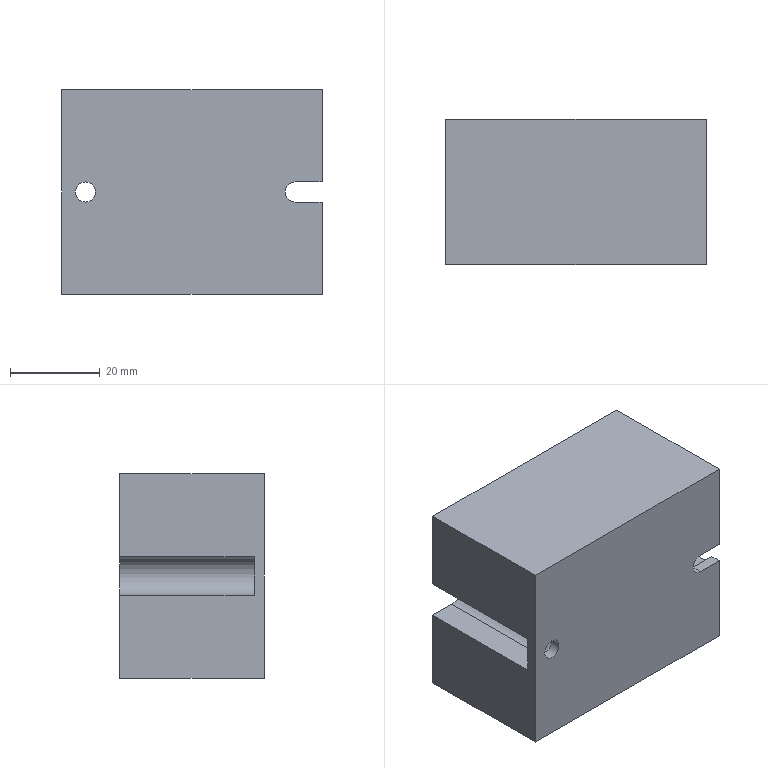Part | NX | features BREP 1 | 1 solid | 19 faces | box 58 x 32.3 x 45.5 mm | volume 80360 mm3 | plane 15 | cylinder 4 | commonest cylinder face diameters 4.5 x2 8.5 x2
STEP:
#1=CARTESIAN_POINT('',(-23.75,2.3,2.25));
#2=VERTEX_POINT('',#1);
#3=CARTESIAN_POINT('',(-23.75,2.3,0.));
#4=DIRECTION('',(0.,1.,0.));
#5=DIRECTION('',(0.,0.,1.));
#6=AXIS2_PLACEMENT_3D('',#3,#4,#5);
#7=CIRCLE('',#6,2.25);
#8=EDGE_CURVE('',#2,#2,#7,.T.);
#9=ORIENTED_EDGE('',*,*,#8,.T.);
#10=EDGE_LOOP('',(#9));
#11=FACE_BOUND('',#10,.T.);
#12=CARTESIAN_POINT('',(-23.75,0.,2.25));
#13=VERTEX_POINT('',#12);
#14=CARTESIAN_POINT('',(-23.75,0.,0.));
#15=DIRECTION('',(0.,1.,0.));
#16=DIRECTION('',(0.,0.,1.));
#17=AXIS2_PLACEMENT_3D('',#14,#15,#16);
#18=CIRCLE('',#17,2.25);
#19=EDGE_CURVE('',#13,#13,#18,.T.);
#20=ORIENTED_EDGE('',*,*,#19,.F.);
#21=EDGE_LOOP('',(#20));
#22=FACE_BOUND('',#21,.T.);
#23=CARTESIAN_POINT('',(-23.75,-27.7,0.));
#24=DIRECTION('',(0.,1.,0.));
#25=DIRECTION('',(0.,0.,1.));
#26=AXIS2_PLACEMENT_3D('',#23,#24,#25);
#27=CYLINDRICAL_SURFACE('',#26,2.25);
#28=ADVANCED_FACE('',(#11,#22),#27,.F.);
#29=CARTESIAN_POINT('',(29.,2.3,-2.25));
#30=VERTEX_POINT('',#29);
#31=CARTESIAN_POINT('',(29.,2.3,-4.25));
#32=VERTEX_POINT('',#31);
#33=CARTESIAN_POINT('',(29.,2.3,-22.75));
#34=DIRECTION('',(0.,0.,-1.));
#35=VECTOR('',#34,1000.);
#36=LINE('',#33,#35);
#37=EDGE_CURVE('',#30,#32,#36,.T.);
#38=ORIENTED_EDGE('',*,*,#37,.F.);
#39=CARTESIAN_POINT('',(29.,0.,-2.25));
#40=VERTEX_POINT('',#39);
#41=CARTESIAN_POINT('',(29.,32.3,-2.25));
#42=DIRECTION('',(0.,-1.,0.));
#43=VECTOR('',#42,1000.);
#44=LINE('',#41,#43);
#45=EDGE_CURVE('',#30,#40,#44,.T.);
#46=ORIENTED_EDGE('',*,*,#45,.T.);
#47=CARTESIAN_POINT('',(29.,0.,-22.75));
#48=VERTEX_POINT('',#47);
#49=CARTESIAN_POINT('',(29.,0.,-22.75));
#50=DIRECTION('',(0.,0.,-1.));
#51=VECTOR('',#50,1000.);
#52=LINE('',#49,#51);
#53=EDGE_CURVE('',#40,#48,#52,.T.);
#54=ORIENTED_EDGE('',*,*,#53,.T.);
#55=CARTESIAN_POINT('',(29.,32.3,-22.75));
#56=VERTEX_POINT('',#55);
#57=CARTESIAN_POINT('',(29.,32.3,-22.75));
#58=DIRECTION('',(0.,-1.,0.));
#59=VECTOR('',#58,1000.);
#60=LINE('',#57,#59);
#61=EDGE_CURVE('',#56,#48,#60,.T.);
#62=ORIENTED_EDGE('',*,*,#61,.F.);
#63=CARTESIAN_POINT('',(29.,32.3,-4.25));
#64=VERTEX_POINT('',#63);
#65=CARTESIAN_POINT('',(29.,32.3,-22.75));
#66=DIRECTION('',(0.,0.,-1.));
#67=VECTOR('',#66,1000.);
#68=LINE('',#65,#67);
#69=EDGE_CURVE('',#64,#56,#68,.T.);
#70=ORIENTED_EDGE('',*,*,#69,.F.);
#71=CARTESIAN_POINT('',(29.,32.3,-4.25));
#72=DIRECTION('',(0.,-1.,0.));
#73=VECTOR('',#72,1000.);
#74=LINE('',#71,#73);
#75=EDGE_CURVE('',#64,#32,#74,.T.);
#76=ORIENTED_EDGE('',*,*,#75,.T.);
#77=EDGE_LOOP('',(#38,#46,#54,#62,#70,#76));
#78=FACE_BOUND('',#77,.T.);
#79=CARTESIAN_POINT('',(29.,32.3,-22.75));
#80=DIRECTION('',(-1.,0.,0.));
#81=DIRECTION('',(0.,0.,1.));
#82=AXIS2_PLACEMENT_3D('',#79,#80,#81);
#83=PLANE('',#82);
#84=ADVANCED_FACE('',(#78),#83,.F.);
#85=CARTESIAN_POINT('',(29.,0.,22.75));
#86=VERTEX_POINT('',#85);
#87=CARTESIAN_POINT('',(29.,0.,2.25));
#88=VERTEX_POINT('',#87);
#89=CARTESIAN_POINT('',(29.,0.,-22.75));
#90=DIRECTION('',(0.,0.,-1.));
#91=VECTOR('',#90,1000.);
#92=LINE('',#89,#91);
#93=EDGE_CURVE('',#86,#88,#92,.T.);
#94=ORIENTED_EDGE('',*,*,#93,.T.);
#95=CARTESIAN_POINT('',(29.,2.3,2.25));
#96=VERTEX_POINT('',#95);
#97=CARTESIAN_POINT('',(29.,32.3,2.25));
#98=DIRECTION('',(0.,1.,0.));
#99=VECTOR('',#98,1000.);
#100=LINE('',#97,#99);
#101=EDGE_CURVE('',#88,#96,#100,.T.);
#102=ORIENTED_EDGE('',*,*,#101,.T.);
#103=CARTESIAN_POINT('',(29.,2.3,4.25));
#104=VERTEX_POINT('',#103);
#105=CARTESIAN_POINT('',(29.,2.3,-22.75));
#106=DIRECTION('',(0.,0.,-1.));
#107=VECTOR('',#106,1000.);
#108=LINE('',#105,#107);
#109=EDGE_CURVE('',#104,#96,#108,.T.);
#110=ORIENTED_EDGE('',*,*,#109,.F.);
#111=CARTESIAN_POINT('',(29.,32.3,4.25));
#112=VERTEX_POINT('',#111);
#113=CARTESIAN_POINT('',(29.,32.3,4.25));
#114=DIRECTION('',(0.,1.,0.));
#115=VECTOR('',#114,1000.);
#116=LINE('',#113,#115);
#117=EDGE_CURVE('',#104,#112,#116,.T.);
#118=ORIENTED_EDGE('',*,*,#117,.T.);
#119=CARTESIAN_POINT('',(29.,32.3,22.75));
#120=VERTEX_POINT('',#119);
#121=CARTESIAN_POINT('',(29.,32.3,-22.75));
#122=DIRECTION('',(0.,0.,-1.));
#123=VECTOR('',#122,1000.);
#124=LINE('',#121,#123);
#125=EDGE_CURVE('',#120,#112,#124,.T.);
#126=ORIENTED_EDGE('',*,*,#125,.F.);
#127=CARTESIAN_POINT('',(29.,32.3,22.75));
#128=DIRECTION('',(0.,-1.,0.));
#129=VECTOR('',#128,1000.);
#130=LINE('',#127,#129);
#131=EDGE_CURVE('',#120,#86,#130,.T.);
#132=ORIENTED_EDGE('',*,*,#131,.T.);
#133=EDGE_LOOP('',(#94,#102,#110,#118,#126,#132));
#134=FACE_BOUND('',#133,.T.);
#135=CARTESIAN_POINT('',(29.,32.3,-22.75));
#136=DIRECTION('',(-1.,0.,0.));
#137=DIRECTION('',(0.,0.,1.));
#138=AXIS2_PLACEMENT_3D('',#135,#136,#137);
#139=PLANE('',#138);
#140=ADVANCED_FACE('',(#134),#139,.F.);
#141=CARTESIAN_POINT('',(-29.,0.,-22.75));
#142=VERTEX_POINT('',#141);
#143=CARTESIAN_POINT('',(-29.,0.,-22.75));
#144=DIRECTION('',(-1.,0.,0.));
#145=VECTOR('',#144,1000.);
#146=LINE('',#143,#145);
#147=EDGE_CURVE('',#48,#142,#146,.T.);
#148=ORIENTED_EDGE('',*,*,#147,.T.);
#149=CARTESIAN_POINT('',(-29.,32.3,-22.75));
#150=VERTEX_POINT('',#149);
#151=CARTESIAN_POINT('',(-29.,32.3,-22.75));
#152=DIRECTION('',(0.,-1.,0.));
#153=VECTOR('',#152,1000.);
#154=LINE('',#151,#153);
#155=EDGE_CURVE('',#150,#142,#154,.T.);
#156=ORIENTED_EDGE('',*,*,#155,.F.);
#157=CARTESIAN_POINT('',(-29.,32.3,-22.75));
#158=DIRECTION('',(-1.,0.,0.));
#159=VECTOR('',#158,1000.);
#160=LINE('',#157,#159);
#161=EDGE_CURVE('',#56,#150,#160,.T.);
#162=ORIENTED_EDGE('',*,*,#161,.F.);
#163=ORIENTED_EDGE('',*,*,#61,.T.);
#164=EDGE_LOOP('',(#148,#156,#162,#163));
#165=FACE_BOUND('',#164,.T.);
#166=CARTESIAN_POINT('',(-29.,32.3,-22.75));
#167=DIRECTION('',(0.,0.,1.));
#168=DIRECTION('',(1.,0.,0.));
#169=AXIS2_PLACEMENT_3D('',#166,#167,#168);
#170=PLANE('',#169);
#171=ADVANCED_FACE('',(#165),#170,.F.);
#172=CARTESIAN_POINT('',(-29.,32.3,4.25));
#173=VERTEX_POINT('',#172);
#174=CARTESIAN_POINT('',(-29.,32.3,22.75));
#175=VERTEX_POINT('',#174);
#176=CARTESIAN_POINT('',(-29.,32.3,-22.75));
#177=DIRECTION('',(0.,0.,1.));
#178=VECTOR('',#177,1000.);
#179=LINE('',#176,#178);
#180=EDGE_CURVE('',#173,#175,#179,.T.);
#181=ORIENTED_EDGE('',*,*,#180,.F.);
#182=CARTESIAN_POINT('',(-29.,2.3,4.25));
#183=VERTEX_POINT('',#182);
#184=CARTESIAN_POINT('',(-29.,32.3,4.25));
#185=DIRECTION('',(0.,-1.,0.));
#186=VECTOR('',#185,1000.);
#187=LINE('',#184,#186);
#188=EDGE_CURVE('',#173,#183,#187,.T.);
#189=ORIENTED_EDGE('',*,*,#188,.T.);
#190=CARTESIAN_POINT('',(-29.,2.3,-4.25));
#191=VERTEX_POINT('',#190);
#192=CARTESIAN_POINT('',(-29.,2.3,-22.75));
#193=DIRECTION('',(0.,0.,-1.));
#194=VECTOR('',#193,1000.);
#195=LINE('',#192,#194);
#196=EDGE_CURVE('',#183,#191,#195,.T.);
#197=ORIENTED_EDGE('',*,*,#196,.T.);
#198=CARTESIAN_POINT('',(-29.,32.3,-4.25));
#199=VERTEX_POINT('',#198);
#200=CARTESIAN_POINT('',(-29.,32.3,-4.25));
#201=DIRECTION('',(0.,1.,0.));
#202=VECTOR('',#201,1000.);
#203=LINE('',#200,#202);
#204=EDGE_CURVE('',#191,#199,#203,.T.);
#205=ORIENTED_EDGE('',*,*,#204,.T.);
#206=CARTESIAN_POINT('',(-29.,32.3,-22.75));
#207=DIRECTION('',(0.,0.,1.));
#208=VECTOR('',#207,1000.);
#209=LINE('',#206,#208);
#210=EDGE_CURVE('',#150,#199,#209,.T.);
#211=ORIENTED_EDGE('',*,*,#210,.F.);
#212=ORIENTED_EDGE('',*,*,#155,.T.);
#213=CARTESIAN_POINT('',(-29.,0.,22.75));
#214=VERTEX_POINT('',#213);
#215=CARTESIAN_POINT('',(-29.,0.,-22.75));
#216=DIRECTION('',(0.,0.,1.));
#217=VECTOR('',#216,1000.);
#218=LINE('',#215,#217);
#219=EDGE_CURVE('',#142,#214,#218,.T.);
#220=ORIENTED_EDGE('',*,*,#219,.T.);
#221=CARTESIAN_POINT('',(-29.,32.3,22.75));
#222=DIRECTION('',(0.,-1.,0.));
#223=VECTOR('',#222,1000.);
#224=LINE('',#221,#223);
#225=EDGE_CURVE('',#175,#214,#224,.T.);
#226=ORIENTED_EDGE('',*,*,#225,.F.);
#227=EDGE_LOOP('',(#181,#189,#197,#205,#211,#212,#220,#226));
#228=FACE_BOUND('',#227,.T.);
#229=CARTESIAN_POINT('',(-29.,32.3,-22.75));
#230=DIRECTION('',(1.,0.,0.));
#231=DIRECTION('',(0.,0.,-1.));
#232=AXIS2_PLACEMENT_3D('',#229,#230,#231);
#233=PLANE('',#232);
#234=ADVANCED_FACE('',(#228),#233,.F.);
#235=CARTESIAN_POINT('',(-29.,0.,22.75));
#236=DIRECTION('',(1.,0.,0.));
#237=VECTOR('',#236,1000.);
#238=LINE('',#235,#237);
#239=EDGE_CURVE('',#214,#86,#238,.T.);
#240=ORIENTED_EDGE('',*,*,#239,.T.);
#241=ORIENTED_EDGE('',*,*,#131,.F.);
#242=CARTESIAN_POINT('',(-29.,32.3,22.75));
#243=DIRECTION('',(1.,0.,0.));
#244=VECTOR('',#243,1000.);
#245=LINE('',#242,#244);
#246=EDGE_CURVE('',#175,#120,#245,.T.);
#247=ORIENTED_EDGE('',*,*,#246,.F.);
#248=ORIENTED_EDGE('',*,*,#225,.T.);
#249=EDGE_LOOP('',(#240,#241,#247,#248));
#250=FACE_BOUND('',#249,.T.);
#251=CARTESIAN_POINT('',(-29.,32.3,22.75));
#252=DIRECTION('',(0.,0.,-1.));
#253=DIRECTION('',(-1.,0.,0.));
#254=AXIS2_PLACEMENT_3D('',#251,#252,#253);
#255=PLANE('',#254);
#256=ADVANCED_FACE('',(#250),#255,.F.);
#257=CARTESIAN_POINT('',(-23.,32.3,4.25));
#258=VERTEX_POINT('',#257);
#259=CARTESIAN_POINT('',(0.,32.3,4.25));
#260=DIRECTION('',(1.,0.,0.));
#261=VECTOR('',#260,1000.);
#262=LINE('',#259,#261);
#263=EDGE_CURVE('',#173,#258,#262,.T.);
#264=ORIENTED_EDGE('',*,*,#263,.F.);
#265=ORIENTED_EDGE('',*,*,#180,.T.);
#266=ORIENTED_EDGE('',*,*,#246,.T.);
#267=ORIENTED_EDGE('',*,*,#125,.T.);
#268=CARTESIAN_POINT('',(23.,32.3,4.25));
#269=VERTEX_POINT('',#268);
#270=CARTESIAN_POINT('',(23.,32.3,4.25));
#271=DIRECTION('',(1.,0.,0.));
#272=VECTOR('',#271,1000.);
#273=LINE('',#270,#272);
#274=EDGE_CURVE('',#269,#112,#273,.T.);
#275=ORIENTED_EDGE('',*,*,#274,.F.);
#276=CARTESIAN_POINT('',(23.,32.3,-4.25));
#277=VERTEX_POINT('',#276);
#278=CARTESIAN_POINT('',(23.,32.3,0.));
#279=DIRECTION('',(0.,1.,0.));
#280=DIRECTION('',(0.,0.,1.));
#281=AXIS2_PLACEMENT_3D('',#278,#279,#280);
#282=CIRCLE('',#281,4.25);
#283=EDGE_CURVE('',#277,#269,#282,.T.);
#284=ORIENTED_EDGE('',*,*,#283,.F.);
#285=CARTESIAN_POINT('',(0.,32.3,-4.25));
#286=DIRECTION('',(-1.,0.,0.));
#287=VECTOR('',#286,1000.);
#288=LINE('',#285,#287);
#289=EDGE_CURVE('',#64,#277,#288,.T.);
#290=ORIENTED_EDGE('',*,*,#289,.F.);
#291=ORIENTED_EDGE('',*,*,#69,.T.);
#292=ORIENTED_EDGE('',*,*,#161,.T.);
#293=ORIENTED_EDGE('',*,*,#210,.T.);
#294=CARTESIAN_POINT('',(-23.,32.3,-4.25));
#295=VERTEX_POINT('',#294);
#296=CARTESIAN_POINT('',(-23.,32.3,-4.25));
#297=DIRECTION('',(-1.,0.,0.));
#298=VECTOR('',#297,1000.);
#299=LINE('',#296,#298);
#300=EDGE_CURVE('',#295,#199,#299,.T.);
#301=ORIENTED_EDGE('',*,*,#300,.F.);
#302=CARTESIAN_POINT('',(-23.,32.3,0.));
#303=DIRECTION('',(0.,1.,0.));
#304=DIRECTION('',(0.,0.,-1.));
#305=AXIS2_PLACEMENT_3D('',#302,#303,#304);
#306=CIRCLE('',#305,4.25);
#307=EDGE_CURVE('',#258,#295,#306,.T.);
#308=ORIENTED_EDGE('',*,*,#307,.F.);
#309=EDGE_LOOP('',(#264,#265,#266,#267,#275,#284,#290,#291,#292,#293,#301,#308));
#310=FACE_BOUND('',#309,.T.);
#311=CARTESIAN_POINT('',(0.,32.3,0.));
#312=DIRECTION('',(0.,1.,0.));
#313=DIRECTION('',(0.,0.,1.));
#314=AXIS2_PLACEMENT_3D('',#311,#312,#313);
#315=PLANE('',#314);
#316=ADVANCED_FACE('',(#310),#315,.T.);
#317=ORIENTED_EDGE('',*,*,#19,.T.);
#318=EDGE_LOOP('',(#317));
#319=FACE_BOUND('',#318,.T.);
#320=ORIENTED_EDGE('',*,*,#53,.F.);
#321=CARTESIAN_POINT('',(23.,0.,-2.25));
#322=VERTEX_POINT('',#321);
#323=CARTESIAN_POINT('',(0.,0.,-2.25));
#324=DIRECTION('',(-1.,0.,0.));
#325=VECTOR('',#324,1000.);
#326=LINE('',#323,#325);
#327=EDGE_CURVE('',#40,#322,#326,.T.);
#328=ORIENTED_EDGE('',*,*,#327,.T.);
#329=CARTESIAN_POINT('',(23.,0.,2.25));
#330=VERTEX_POINT('',#329);
#331=CARTESIAN_POINT('',(23.,0.,0.));
#332=DIRECTION('',(0.,1.,0.));
#333=DIRECTION('',(0.,0.,1.));
#334=AXIS2_PLACEMENT_3D('',#331,#332,#333);
#335=CIRCLE('',#334,2.25);
#336=EDGE_CURVE('',#322,#330,#335,.T.);
#337=ORIENTED_EDGE('',*,*,#336,.T.);
#338=CARTESIAN_POINT('',(0.,0.,2.25));
#339=DIRECTION('',(1.,0.,0.));
#340=VECTOR('',#339,1000.);
#341=LINE('',#338,#340);
#342=EDGE_CURVE('',#330,#88,#341,.T.);
#343=ORIENTED_EDGE('',*,*,#342,.T.);
#344=ORIENTED_EDGE('',*,*,#93,.F.);
#345=ORIENTED_EDGE('',*,*,#239,.F.);
#346=ORIENTED_EDGE('',*,*,#219,.F.);
#347=ORIENTED_EDGE('',*,*,#147,.F.);
#348=EDGE_LOOP('',(#320,#328,#337,#343,#344,#345,#346,#347));
#349=FACE_BOUND('',#348,.T.);
#350=CARTESIAN_POINT('',(0.,0.,0.));
#351=DIRECTION('',(0.,1.,0.));
#352=DIRECTION('',(0.,0.,1.));
#353=AXIS2_PLACEMENT_3D('',#350,#351,#352);
#354=PLANE('',#353);
#355=ADVANCED_FACE('',(#319,#349),#354,.F.);
#356=CARTESIAN_POINT('',(23.,2.3,-2.25));
#357=VERTEX_POINT('',#356);
#358=CARTESIAN_POINT('',(23.,2.3,-2.25));
#359=DIRECTION('',(-1.,0.,0.));
#360=VECTOR('',#359,1000.);
#361=LINE('',#358,#360);
#362=EDGE_CURVE('',#30,#357,#361,.T.);
#363=ORIENTED_EDGE('',*,*,#362,.F.);
#364=ORIENTED_EDGE('',*,*,#37,.T.);
#365=CARTESIAN_POINT('',(23.,2.3,-4.25));
#366=VERTEX_POINT('',#365);
#367=CARTESIAN_POINT('',(23.,2.3,-4.25));
#368=DIRECTION('',(-1.,0.,0.));
#369=VECTOR('',#368,1000.);
#370=LINE('',#367,#369);
#371=EDGE_CURVE('',#32,#366,#370,.T.);
#372=ORIENTED_EDGE('',*,*,#371,.T.);
#373=CARTESIAN_POINT('',(23.,2.3,4.25));
#374=VERTEX_POINT('',#373);
#375=CARTESIAN_POINT('',(23.,2.3,0.));
#376=DIRECTION('',(0.,1.,0.));
#377=DIRECTION('',(0.,0.,1.));
#378=AXIS2_PLACEMENT_3D('',#375,#376,#377);
#379=CIRCLE('',#378,4.25);
#380=EDGE_CURVE('',#366,#374,#379,.T.);
#381=ORIENTED_EDGE('',*,*,#380,.T.);
#382=CARTESIAN_POINT('',(23.,2.3,4.25));
#383=DIRECTION('',(1.,0.,0.));
#384=VECTOR('',#383,1000.);
#385=LINE('',#382,#384);
#386=EDGE_CURVE('',#374,#104,#385,.T.);
#387=ORIENTED_EDGE('',*,*,#386,.T.);
#388=ORIENTED_EDGE('',*,*,#109,.T.);
#389=CARTESIAN_POINT('',(23.,2.3,2.25));
#390=VERTEX_POINT('',#389);
#391=CARTESIAN_POINT('',(23.,2.3,2.25));
#392=DIRECTION('',(1.,0.,0.));
#393=VECTOR('',#392,1000.);
#394=LINE('',#391,#393);
#395=EDGE_CURVE('',#390,#96,#394,.T.);
#396=ORIENTED_EDGE('',*,*,#395,.F.);
#397=CARTESIAN_POINT('',(23.,2.3,0.));
#398=DIRECTION('',(0.,1.,0.));
#399=DIRECTION('',(0.,0.,1.));
#400=AXIS2_PLACEMENT_3D('',#397,#398,#399);
#401=CIRCLE('',#400,2.25);
#402=EDGE_CURVE('',#357,#390,#401,.T.);
#403=ORIENTED_EDGE('',*,*,#402,.F.);
#404=EDGE_LOOP('',(#363,#364,#372,#381,#387,#388,#396,#403));
#405=FACE_BOUND('',#404,.T.);
#406=CARTESIAN_POINT('',(23.,2.3,0.));
#407=DIRECTION('',(0.,1.,0.));
#408=DIRECTION('',(0.,0.,1.));
#409=AXIS2_PLACEMENT_3D('',#406,#407,#408);
#410=PLANE('',#409);
#411=ADVANCED_FACE('',(#405),#410,.T.);
#412=ORIENTED_EDGE('',*,*,#289,.T.);
#413=CARTESIAN_POINT('',(23.,2.3,-4.25));
#414=DIRECTION('',(0.,1.,0.));
#415=VECTOR('',#414,1000.);
#416=LINE('',#413,#415);
#417=EDGE_CURVE('',#366,#277,#416,.T.);
#418=ORIENTED_EDGE('',*,*,#417,.F.);
#419=ORIENTED_EDGE('',*,*,#371,.F.);
#420=ORIENTED_EDGE('',*,*,#75,.F.);
#421=EDGE_LOOP('',(#412,#418,#419,#420));
#422=FACE_BOUND('',#421,.T.);
#423=CARTESIAN_POINT('',(23.,2.3,-4.25));
#424=DIRECTION('',(0.,0.,-1.));
#425=DIRECTION('',(-1.,0.,0.));
#426=AXIS2_PLACEMENT_3D('',#423,#424,#425);
#427=PLANE('',#426);
#428=ADVANCED_FACE('',(#422),#427,.F.);
#429=ORIENTED_EDGE('',*,*,#386,.F.);
#430=CARTESIAN_POINT('',(23.,2.3,4.25));
#431=DIRECTION('',(0.,1.,0.));
#432=VECTOR('',#431,1000.);
#433=LINE('',#430,#432);
#434=EDGE_CURVE('',#374,#269,#433,.T.);
#435=ORIENTED_EDGE('',*,*,#434,.T.);
#436=ORIENTED_EDGE('',*,*,#274,.T.);
#437=ORIENTED_EDGE('',*,*,#117,.F.);
#438=EDGE_LOOP('',(#429,#435,#436,#437));
#439=FACE_BOUND('',#438,.T.);
#440=CARTESIAN_POINT('',(23.,2.3,4.25));
#441=DIRECTION('',(0.,0.,1.));
#442=DIRECTION('',(1.,0.,0.));
#443=AXIS2_PLACEMENT_3D('',#440,#441,#442);
#444=PLANE('',#443);
#445=ADVANCED_FACE('',(#439),#444,.F.);
#446=ORIENTED_EDGE('',*,*,#283,.T.);
#447=ORIENTED_EDGE('',*,*,#434,.F.);
#448=ORIENTED_EDGE('',*,*,#380,.F.);
#449=ORIENTED_EDGE('',*,*,#417,.T.);
#450=EDGE_LOOP('',(#446,#447,#448,#449));
#451=FACE_BOUND('',#450,.T.);
#452=CARTESIAN_POINT('',(23.,2.3,0.));
#453=DIRECTION('',(0.,1.,0.));
#454=DIRECTION('',(0.,0.,1.));
#455=AXIS2_PLACEMENT_3D('',#452,#453,#454);
#456=CYLINDRICAL_SURFACE('',#455,4.25);
#457=ADVANCED_FACE('',(#451),#456,.F.);
#458=ORIENTED_EDGE('',*,*,#8,.F.);
#459=EDGE_LOOP('',(#458));
#460=FACE_BOUND('',#459,.T.);
#461=CARTESIAN_POINT('',(-23.,2.3,4.25));
#462=VERTEX_POINT('',#461);
#463=CARTESIAN_POINT('',(-23.,2.3,4.25));
#464=DIRECTION('',(1.,0.,0.));
#465=VECTOR('',#464,1000.);
#466=LINE('',#463,#465);
#467=EDGE_CURVE('',#183,#462,#466,.T.);
#468=ORIENTED_EDGE('',*,*,#467,.T.);
#469=CARTESIAN_POINT('',(-23.,2.3,-4.25));
#470=VERTEX_POINT('',#469);
#471=CARTESIAN_POINT('',(-23.,2.3,0.));
#472=DIRECTION('',(0.,1.,0.));
#473=DIRECTION('',(0.,0.,-1.));
#474=AXIS2_PLACEMENT_3D('',#471,#472,#473);
#475=CIRCLE('',#474,4.25);
#476=EDGE_CURVE('',#462,#470,#475,.T.);
#477=ORIENTED_EDGE('',*,*,#476,.T.);
#478=CARTESIAN_POINT('',(-23.,2.3,-4.25));
#479=DIRECTION('',(-1.,0.,0.));
#480=VECTOR('',#479,1000.);
#481=LINE('',#478,#480);
#482=EDGE_CURVE('',#470,#191,#481,.T.);
#483=ORIENTED_EDGE('',*,*,#482,.T.);
#484=ORIENTED_EDGE('',*,*,#196,.F.);
#485=EDGE_LOOP('',(#468,#477,#483,#484));
#486=FACE_BOUND('',#485,.T.);
#487=CARTESIAN_POINT('',(-23.,2.3,0.));
#488=DIRECTION('',(0.,-1.,0.));
#489=DIRECTION('',(0.,0.,-1.));
#490=AXIS2_PLACEMENT_3D('',#487,#488,#489);
#491=PLANE('',#490);
#492=ADVANCED_FACE('',(#460,#486),#491,.F.);
#493=ORIENTED_EDGE('',*,*,#263,.T.);
#494=CARTESIAN_POINT('',(-23.,2.3,4.25));
#495=DIRECTION('',(0.,1.,0.));
#496=VECTOR('',#495,1000.);
#497=LINE('',#494,#496);
#498=EDGE_CURVE('',#462,#258,#497,.T.);
#499=ORIENTED_EDGE('',*,*,#498,.F.);
#500=ORIENTED_EDGE('',*,*,#467,.F.);
#501=ORIENTED_EDGE('',*,*,#188,.F.);
#502=EDGE_LOOP('',(#493,#499,#500,#501));
#503=FACE_BOUND('',#502,.T.);
#504=CARTESIAN_POINT('',(-23.,2.3,4.25));
#505=DIRECTION('',(0.,0.,1.));
#506=DIRECTION('',(1.,0.,0.));
#507=AXIS2_PLACEMENT_3D('',#504,#505,#506);
#508=PLANE('',#507);
#509=ADVANCED_FACE('',(#503),#508,.F.);
#510=ORIENTED_EDGE('',*,*,#482,.F.);
#511=CARTESIAN_POINT('',(-23.,2.3,-4.25));
#512=DIRECTION('',(0.,1.,0.));
#513=VECTOR('',#512,1000.);
#514=LINE('',#511,#513);
#515=EDGE_CURVE('',#470,#295,#514,.T.);
#516=ORIENTED_EDGE('',*,*,#515,.T.);
#517=ORIENTED_EDGE('',*,*,#300,.T.);
#518=ORIENTED_EDGE('',*,*,#204,.F.);
#519=EDGE_LOOP('',(#510,#516,#517,#518));
#520=FACE_BOUND('',#519,.T.);
#521=CARTESIAN_POINT('',(-23.,2.3,-4.25));
#522=DIRECTION('',(0.,0.,-1.));
#523=DIRECTION('',(-1.,0.,0.));
#524=AXIS2_PLACEMENT_3D('',#521,#522,#523);
#525=PLANE('',#524);
#526=ADVANCED_FACE('',(#520),#525,.F.);
#527=ORIENTED_EDGE('',*,*,#307,.T.);
#528=ORIENTED_EDGE('',*,*,#515,.F.);
#529=ORIENTED_EDGE('',*,*,#476,.F.);
#530=ORIENTED_EDGE('',*,*,#498,.T.);
#531=EDGE_LOOP('',(#527,#528,#529,#530));
#532=FACE_BOUND('',#531,.T.);
#533=CARTESIAN_POINT('',(-23.,2.3,0.));
#534=DIRECTION('',(0.,1.,0.));
#535=DIRECTION('',(0.,0.,1.));
#536=AXIS2_PLACEMENT_3D('',#533,#534,#535);
#537=CYLINDRICAL_SURFACE('',#536,4.25);
#538=ADVANCED_FACE('',(#532),#537,.F.);
#539=CARTESIAN_POINT('',(23.,-27.7,-2.25));
#540=DIRECTION('',(0.,1.,0.));
#541=VECTOR('',#540,1000.);
#542=LINE('',#539,#541);
#543=EDGE_CURVE('',#322,#357,#542,.T.);
#544=ORIENTED_EDGE('',*,*,#543,.T.);
#545=ORIENTED_EDGE('',*,*,#402,.T.);
#546=CARTESIAN_POINT('',(23.,-27.7,2.25));
#547=DIRECTION('',(0.,1.,0.));
#548=VECTOR('',#547,1000.);
#549=LINE('',#546,#548);
#550=EDGE_CURVE('',#330,#390,#549,.T.);
#551=ORIENTED_EDGE('',*,*,#550,.F.);
#552=ORIENTED_EDGE('',*,*,#336,.F.);
#553=EDGE_LOOP('',(#544,#545,#551,#552));
#554=FACE_BOUND('',#553,.T.);
#555=CARTESIAN_POINT('',(23.,-27.7,0.));
#556=DIRECTION('',(0.,1.,0.));
#557=DIRECTION('',(0.,0.,1.));
#558=AXIS2_PLACEMENT_3D('',#555,#556,#557);
#559=CYLINDRICAL_SURFACE('',#558,2.25);
#560=ADVANCED_FACE('',(#554),#559,.F.);
#561=ORIENTED_EDGE('',*,*,#362,.T.);
#562=ORIENTED_EDGE('',*,*,#543,.F.);
#563=ORIENTED_EDGE('',*,*,#327,.F.);
#564=ORIENTED_EDGE('',*,*,#45,.F.);
#565=EDGE_LOOP('',(#561,#562,#563,#564));
#566=FACE_BOUND('',#565,.T.);
#567=CARTESIAN_POINT('',(23.,-27.7,-2.25));
#568=DIRECTION('',(0.,0.,-1.));
#569=DIRECTION('',(-1.,0.,0.));
#570=AXIS2_PLACEMENT_3D('',#567,#568,#569);
#571=PLANE('',#570);
#572=ADVANCED_FACE('',(#566),#571,.F.);
#573=ORIENTED_EDGE('',*,*,#342,.F.);
#574=ORIENTED_EDGE('',*,*,#550,.T.);
#575=ORIENTED_EDGE('',*,*,#395,.T.);
#576=ORIENTED_EDGE('',*,*,#101,.F.);
#577=EDGE_LOOP('',(#573,#574,#575,#576));
#578=FACE_BOUND('',#577,.T.);
#579=CARTESIAN_POINT('',(23.,-27.7,2.25));
#580=DIRECTION('',(0.,0.,1.));
#581=DIRECTION('',(1.,0.,0.));
#582=AXIS2_PLACEMENT_3D('',#579,#580,#581);
#583=PLANE('',#582);
#584=ADVANCED_FACE('',(#578),#583,.F.);
#585=CLOSED_SHELL('',(#28,#84,#140,#171,#234,#256,#316,#355,#411,#428,#445,#457,#492,#509,#526,#538,#560,#572,#584));
#586=MANIFOLD_SOLID_BREP('',#585);
#587=(LENGTH_UNIT()NAMED_UNIT(*)SI_UNIT(.MILLI.,.METRE.));
#588=UNCERTAINTY_MEASURE_WITH_UNIT(LENGTH_MEASURE(0.00001),#587,'','');
#589=(NAMED_UNIT(*)PLANE_ANGLE_UNIT()SI_UNIT($,.RADIAN.));
#590=(NAMED_UNIT(*)SI_UNIT($,.STERADIAN.)SOLID_ANGLE_UNIT());
#591=(GEOMETRIC_REPRESENTATION_CONTEXT(3)GLOBAL_UNCERTAINTY_ASSIGNED_CONTEXT((#588))GLOBAL_UNIT_ASSIGNED_CONTEXT((#587,#589,#590))REPRESENTATION_CONTEXT('',''));
#592=ADVANCED_BREP_SHAPE_REPRESENTATION('',(#586),#591);